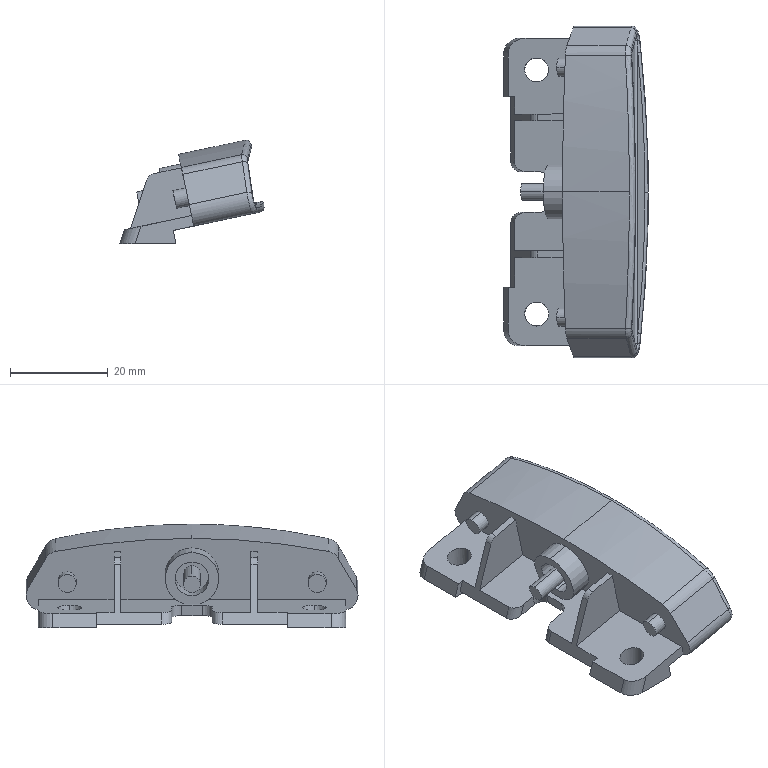Part | SolidWorks | features BaseBody 1 | 1 solid | 103 faces | box 29.6 x 68.008 x 21.238 mm | volume 14301 mm3 | plane 38 | cylinder 35 | spline 20 | torus 6 | cone 4 | commonest cylinder face diameters 4 x6 6 x6 1 x4 3.7 x4 4.9 x4 3.5 x2